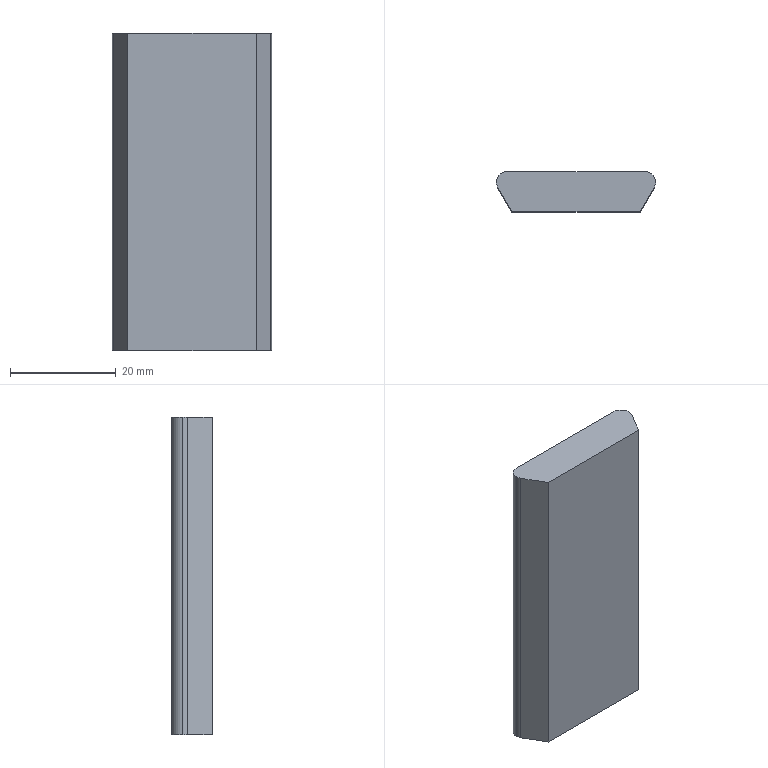Part | STEP file | 101000007812 | 1 solid | 10 faces | box 30.072 x 7.6 x 60 mm | volume 12718 mm3 | plane 6 | cylinder 4 | commonest cylinder face diameters 4 x4
STEP:
#1=CARTESIAN_POINT('',(10.458,8.,60.));
#2=VERTEX_POINT('',#1);
#3=CARTESIAN_POINT('',(10.726,7.,60.));
#4=VERTEX_POINT('',#3);
#5=CARTESIAN_POINT('',(12.458,8.,60.));
#6=DIRECTION('',(0.,0.,-1.));
#7=AXIS2_PLACEMENT_3D('',#5,#6,$);
#8=CIRCLE('',#7,2.);
#9=EDGE_CURVE('',#2,#4,#8,.F.);
#10=ORIENTED_EDGE('',*,*,#9,.F.);
#11=CARTESIAN_POINT('',(10.458,8.,0.));
#12=VERTEX_POINT('',#11);
#13=CARTESIAN_POINT('',(10.458,8.,60.));
#14=DIRECTION('',(0.,0.,-1.));
#15=VECTOR('',#14,1.);
#16=LINE('',#13,#15);
#17=EDGE_CURVE('',#2,#12,#16,.T.);
#18=ORIENTED_EDGE('',*,*,#17,.T.);
#19=CARTESIAN_POINT('',(10.726,7.,0.));
#20=VERTEX_POINT('',#19);
#21=CARTESIAN_POINT('',(12.458,8.,0.));
#22=DIRECTION('',(0.,0.,-1.));
#23=AXIS2_PLACEMENT_3D('',#21,#22,$);
#24=CIRCLE('',#23,2.);
#25=EDGE_CURVE('',#20,#12,#24,.T.);
#26=ORIENTED_EDGE('',*,*,#25,.F.);
#27=CARTESIAN_POINT('',(10.726,7.,60.));
#28=DIRECTION('',(0.,0.,-1.));
#29=VECTOR('',#28,1.);
#30=LINE('',#27,#29);
#31=EDGE_CURVE('',#4,#20,#30,.T.);
#32=ORIENTED_EDGE('',*,*,#31,.F.);
#33=EDGE_LOOP('',(#10,#18,#26,#32));
#34=FACE_OUTER_BOUND('',#33,.T.);
#35=CARTESIAN_POINT('',(12.458,8.,60.));
#36=DIRECTION('',(0.,0.,-1.));
#37=DIRECTION('',(1.,0.,0.));
#38=AXIS2_PLACEMENT_3D('',#35,#36,#37);
#39=CYLINDRICAL_SURFACE('',#38,2.);
#40=ADVANCED_FACE('',(#34),#39,.T.);
#41=CARTESIAN_POINT('',(37.606,2.4,60.));
#42=VERTEX_POINT('',#41);
#43=CARTESIAN_POINT('',(13.382,2.4,60.));
#44=VERTEX_POINT('',#43);
#45=CARTESIAN_POINT('',(25.494,2.4,60.));
#46=DIRECTION('',(-1.,0.,0.));
#47=VECTOR('',#46,1.);
#48=LINE('',#45,#47);
#49=EDGE_CURVE('',#42,#44,#48,.T.);
#50=ORIENTED_EDGE('',*,*,#49,.F.);
#51=CARTESIAN_POINT('',(40.262,7.,60.));
#52=VERTEX_POINT('',#51);
#53=CARTESIAN_POINT('',(38.934,4.7,60.));
#54=DIRECTION('',(0.5,0.866,0.));
#55=VECTOR('',#54,1.);
#56=LINE('',#53,#55);
#57=EDGE_CURVE('',#42,#52,#56,.T.);
#58=ORIENTED_EDGE('',*,*,#57,.T.);
#59=CARTESIAN_POINT('',(40.53,8.,60.));
#60=VERTEX_POINT('',#59);
#61=CARTESIAN_POINT('',(38.53,8.,60.));
#62=DIRECTION('',(0.,0.,1.));
#63=AXIS2_PLACEMENT_3D('',#61,#62,$);
#64=CIRCLE('',#63,2.);
#65=EDGE_CURVE('',#52,#60,#64,.T.);
#66=ORIENTED_EDGE('',*,*,#65,.T.);
#67=CARTESIAN_POINT('',(38.53,10.,60.));
#68=VERTEX_POINT('',#67);
#69=CARTESIAN_POINT('',(38.53,8.,60.));
#70=DIRECTION('',(0.,0.,1.));
#71=AXIS2_PLACEMENT_3D('',#69,#70,$);
#72=CIRCLE('',#71,2.);
#73=EDGE_CURVE('',#60,#68,#72,.T.);
#74=ORIENTED_EDGE('',*,*,#73,.T.);
#75=CARTESIAN_POINT('',(12.458,10.,60.));
#76=VERTEX_POINT('',#75);
#77=CARTESIAN_POINT('',(25.494,10.,60.));
#78=DIRECTION('',(-1.,0.,0.));
#79=VECTOR('',#78,1.);
#80=LINE('',#77,#79);
#81=EDGE_CURVE('',#68,#76,#80,.T.);
#82=ORIENTED_EDGE('',*,*,#81,.T.);
#83=CARTESIAN_POINT('',(12.458,8.,60.));
#84=DIRECTION('',(0.,0.,1.));
#85=AXIS2_PLACEMENT_3D('',#83,#84,$);
#86=CIRCLE('',#85,2.);
#87=EDGE_CURVE('',#76,#2,#86,.T.);
#88=ORIENTED_EDGE('',*,*,#87,.T.);
#89=ORIENTED_EDGE('',*,*,#9,.T.);
#90=CARTESIAN_POINT('',(12.054,4.7,60.));
#91=DIRECTION('',(0.5,-0.866,0.));
#92=VECTOR('',#91,1.);
#93=LINE('',#90,#92);
#94=EDGE_CURVE('',#4,#44,#93,.T.);
#95=ORIENTED_EDGE('',*,*,#94,.T.);
#96=EDGE_LOOP('',(#50,#58,#66,#74,#82,#88,#89,#95));
#97=FACE_OUTER_BOUND('',#96,.T.);
#98=CARTESIAN_POINT('',(36.22,0.,60.));
#99=DIRECTION('',(0.,0.,1.));
#100=DIRECTION('',(1.,0.,0.));
#101=AXIS2_PLACEMENT_3D('',#98,#99,#100);
#102=PLANE('',#101);
#103=ADVANCED_FACE('',(#97),#102,.T.);
#104=ORIENTED_EDGE('',*,*,#17,.F.);
#105=ORIENTED_EDGE('',*,*,#87,.F.);
#106=CARTESIAN_POINT('',(12.458,10.,0.));
#107=VERTEX_POINT('',#106);
#108=CARTESIAN_POINT('',(12.458,10.,60.));
#109=DIRECTION('',(0.,0.,-1.));
#110=VECTOR('',#109,1.);
#111=LINE('',#108,#110);
#112=EDGE_CURVE('',#107,#76,#111,.F.);
#113=ORIENTED_EDGE('',*,*,#112,.F.);
#114=CARTESIAN_POINT('',(12.458,8.,0.));
#115=DIRECTION('',(0.,0.,-1.));
#116=AXIS2_PLACEMENT_3D('',#114,#115,$);
#117=CIRCLE('',#116,2.);
#118=EDGE_CURVE('',#12,#107,#117,.T.);
#119=ORIENTED_EDGE('',*,*,#118,.F.);
#120=EDGE_LOOP('',(#104,#105,#113,#119));
#121=FACE_OUTER_BOUND('',#120,.T.);
#122=CARTESIAN_POINT('',(12.458,8.,60.));
#123=DIRECTION('',(0.,0.,-1.));
#124=DIRECTION('',(-1.,0.,0.));
#125=AXIS2_PLACEMENT_3D('',#122,#123,#124);
#126=CYLINDRICAL_SURFACE('',#125,2.);
#127=ADVANCED_FACE('',(#121),#126,.T.);
#128=CARTESIAN_POINT('',(37.606,2.4,0.));
#129=VERTEX_POINT('',#128);
#130=CARTESIAN_POINT('',(40.262,7.,0.));
#131=VERTEX_POINT('',#130);
#132=CARTESIAN_POINT('',(38.934,4.7,0.));
#133=DIRECTION('',(0.5,0.866,0.));
#134=VECTOR('',#133,1.);
#135=LINE('',#132,#134);
#136=EDGE_CURVE('',#129,#131,#135,.T.);
#137=ORIENTED_EDGE('',*,*,#136,.F.);
#138=CARTESIAN_POINT('',(13.382,2.4,0.));
#139=VERTEX_POINT('',#138);
#140=CARTESIAN_POINT('',(25.494,2.4,0.));
#141=DIRECTION('',(-1.,0.,0.));
#142=VECTOR('',#141,1.);
#143=LINE('',#140,#142);
#144=EDGE_CURVE('',#129,#139,#143,.T.);
#145=ORIENTED_EDGE('',*,*,#144,.T.);
#146=CARTESIAN_POINT('',(12.054,4.7,0.));
#147=DIRECTION('',(0.5,-0.866,0.));
#148=VECTOR('',#147,1.);
#149=LINE('',#146,#148);
#150=EDGE_CURVE('',#20,#139,#149,.T.);
#151=ORIENTED_EDGE('',*,*,#150,.F.);
#152=ORIENTED_EDGE('',*,*,#25,.T.);
#153=ORIENTED_EDGE('',*,*,#118,.T.);
#154=CARTESIAN_POINT('',(38.53,10.,0.));
#155=VERTEX_POINT('',#154);
#156=CARTESIAN_POINT('',(25.494,10.,0.));
#157=DIRECTION('',(-1.,0.,0.));
#158=VECTOR('',#157,1.);
#159=LINE('',#156,#158);
#160=EDGE_CURVE('',#155,#107,#159,.T.);
#161=ORIENTED_EDGE('',*,*,#160,.F.);
#162=CARTESIAN_POINT('',(40.53,8.,0.));
#163=VERTEX_POINT('',#162);
#164=CARTESIAN_POINT('',(38.53,10.,0.));
#165=CARTESIAN_POINT('',(38.737,10.,0.));
#166=CARTESIAN_POINT('',(38.945,9.973,0.));
#167=CARTESIAN_POINT('',(39.148,9.919,0.));
#168=CARTESIAN_POINT('',(39.536,9.759,0.));
#169=CARTESIAN_POINT('',(39.87,9.506,0.));
#170=CARTESIAN_POINT('',(40.02,9.358,0.));
#171=CARTESIAN_POINT('',(40.277,9.027,0.));
#172=CARTESIAN_POINT('',(40.441,8.642,0.));
#173=CARTESIAN_POINT('',(40.498,8.439,0.));
#174=CARTESIAN_POINT('',(40.528,8.227,0.));
#175=CARTESIAN_POINT('',(40.53,8.014,0.));
#176=CARTESIAN_POINT('',(40.53,8.01,0.));
#177=CARTESIAN_POINT('',(40.53,8.005,0.));
#178=CARTESIAN_POINT('',(40.53,8.,0.));
#179=B_SPLINE_CURVE_WITH_KNOTS('',5,(#164,#165,#166,#167,#168,#169,#170,#171,#172,#173,#174,#175,#176,#177,#178),.UNSPECIFIED.,.F.,.U.,(6,3,3,3,6),(0.,1.47,2.939,4.409,4.443),.UNSPECIFIED.);
#180=EDGE_CURVE('',#155,#163,#179,.T.);
#181=ORIENTED_EDGE('',*,*,#180,.T.);
#182=CARTESIAN_POINT('',(40.53,8.,0.));
#183=CARTESIAN_POINT('',(40.53,7.797,0.));
#184=CARTESIAN_POINT('',(40.504,7.594,0.));
#185=CARTESIAN_POINT('',(40.452,7.395,0.));
#186=CARTESIAN_POINT('',(40.374,7.199,0.));
#187=CARTESIAN_POINT('',(40.271,7.017,0.));
#188=CARTESIAN_POINT('',(40.268,7.011,0.));
#189=CARTESIAN_POINT('',(40.265,7.006,0.));
#190=CARTESIAN_POINT('',(40.262,7.,0.));
#191=B_SPLINE_CURVE_WITH_KNOTS('',5,(#182,#183,#184,#185,#186,#187,#188,#189,#190),.UNSPECIFIED.,.F.,.U.,(6,3,6),(4.443,5.879,5.924),.UNSPECIFIED.);
#192=EDGE_CURVE('',#163,#131,#191,.T.);
#193=ORIENTED_EDGE('',*,*,#192,.T.);
#194=EDGE_LOOP('',(#137,#145,#151,#152,#153,#161,#181,#193));
#195=FACE_OUTER_BOUND('',#194,.T.);
#196=CARTESIAN_POINT('',(36.22,0.,0.));
#197=DIRECTION('',(0.,0.,1.));
#198=DIRECTION('',(1.,0.,0.));
#199=AXIS2_PLACEMENT_3D('',#196,#197,#198);
#200=PLANE('',#199);
#201=ADVANCED_FACE('',(#195),#200,.F.);
#202=ORIENTED_EDGE('',*,*,#150,.T.);
#203=CARTESIAN_POINT('',(13.382,2.4,30.));
#204=DIRECTION('',(0.,0.,1.));
#205=VECTOR('',#204,1.);
#206=LINE('',#203,#205);
#207=EDGE_CURVE('',#139,#44,#206,.T.);
#208=ORIENTED_EDGE('',*,*,#207,.T.);
#209=ORIENTED_EDGE('',*,*,#94,.F.);
#210=ORIENTED_EDGE('',*,*,#31,.T.);
#211=EDGE_LOOP('',(#202,#208,#209,#210));
#212=FACE_OUTER_BOUND('',#211,.T.);
#213=CARTESIAN_POINT('',(14.767,0.,60.));
#214=DIRECTION('',(0.866,0.5,0.));
#215=DIRECTION('',(-0.5,0.866,0.));
#216=AXIS2_PLACEMENT_3D('',#213,#214,#215);
#217=PLANE('',#216);
#218=ADVANCED_FACE('',(#212),#217,.F.);
#219=ORIENTED_EDGE('',*,*,#49,.T.);
#220=ORIENTED_EDGE('',*,*,#207,.F.);
#221=ORIENTED_EDGE('',*,*,#144,.F.);
#222=CARTESIAN_POINT('',(37.606,2.4,30.));
#223=DIRECTION('',(0.,0.,-1.));
#224=VECTOR('',#223,1.);
#225=LINE('',#222,#224);
#226=EDGE_CURVE('',#42,#129,#225,.T.);
#227=ORIENTED_EDGE('',*,*,#226,.F.);
#228=EDGE_LOOP('',(#219,#220,#221,#227));
#229=FACE_OUTER_BOUND('',#228,.T.);
#230=CARTESIAN_POINT('',(10.494,2.4,0.));
#231=DIRECTION('',(0.,1.,0.));
#232=DIRECTION('',(-1.,0.,0.));
#233=AXIS2_PLACEMENT_3D('',#230,#231,#232);
#234=PLANE('',#233);
#235=ADVANCED_FACE('',(#229),#234,.F.);
#236=ORIENTED_EDGE('',*,*,#57,.F.);
#237=ORIENTED_EDGE('',*,*,#226,.T.);
#238=ORIENTED_EDGE('',*,*,#136,.T.);
#239=CARTESIAN_POINT('',(40.262,7.,30.));
#240=DIRECTION('',(0.,0.,1.));
#241=VECTOR('',#240,1.);
#242=LINE('',#239,#241);
#243=EDGE_CURVE('',#131,#52,#242,.T.);
#244=ORIENTED_EDGE('',*,*,#243,.T.);
#245=EDGE_LOOP('',(#236,#237,#238,#244));
#246=FACE_OUTER_BOUND('',#245,.T.);
#247=CARTESIAN_POINT('',(36.22,0.,60.));
#248=DIRECTION('',(-0.866,0.5,0.));
#249=DIRECTION('',(-0.5,-0.866,0.));
#250=AXIS2_PLACEMENT_3D('',#247,#248,#249);
#251=PLANE('',#250);
#252=ADVANCED_FACE('',(#246),#251,.F.);
#253=CARTESIAN_POINT('',(40.53,8.,60.));
#254=DIRECTION('',(0.,0.,-1.));
#255=VECTOR('',#254,1.);
#256=LINE('',#253,#255);
#257=EDGE_CURVE('',#60,#163,#256,.T.);
#258=ORIENTED_EDGE('',*,*,#257,.F.);
#259=ORIENTED_EDGE('',*,*,#65,.F.);
#260=ORIENTED_EDGE('',*,*,#243,.F.);
#261=ORIENTED_EDGE('',*,*,#192,.F.);
#262=EDGE_LOOP('',(#258,#259,#260,#261));
#263=FACE_OUTER_BOUND('',#262,.T.);
#264=CARTESIAN_POINT('',(38.53,8.,60.));
#265=DIRECTION('',(0.,0.,-1.));
#266=DIRECTION('',(1.,0.,0.));
#267=AXIS2_PLACEMENT_3D('',#264,#265,#266);
#268=CYLINDRICAL_SURFACE('',#267,2.);
#269=ADVANCED_FACE('',(#263),#268,.T.);
#270=ORIENTED_EDGE('',*,*,#257,.T.);
#271=ORIENTED_EDGE('',*,*,#180,.F.);
#272=CARTESIAN_POINT('',(38.53,10.,60.));
#273=DIRECTION('',(0.,0.,-1.));
#274=VECTOR('',#273,1.);
#275=LINE('',#272,#274);
#276=EDGE_CURVE('',#68,#155,#275,.T.);
#277=ORIENTED_EDGE('',*,*,#276,.F.);
#278=ORIENTED_EDGE('',*,*,#73,.F.);
#279=EDGE_LOOP('',(#270,#271,#277,#278));
#280=FACE_OUTER_BOUND('',#279,.T.);
#281=CARTESIAN_POINT('',(38.53,8.,60.));
#282=DIRECTION('',(0.,0.,-1.));
#283=DIRECTION('',(-1.,0.,0.));
#284=AXIS2_PLACEMENT_3D('',#281,#282,#283);
#285=CYLINDRICAL_SURFACE('',#284,2.);
#286=ADVANCED_FACE('',(#280),#285,.T.);
#287=ORIENTED_EDGE('',*,*,#81,.F.);
#288=ORIENTED_EDGE('',*,*,#276,.T.);
#289=ORIENTED_EDGE('',*,*,#160,.T.);
#290=ORIENTED_EDGE('',*,*,#112,.T.);
#291=EDGE_LOOP('',(#287,#288,#289,#290));
#292=FACE_OUTER_BOUND('',#291,.T.);
#293=CARTESIAN_POINT('',(8.994,10.,60.));
#294=DIRECTION('',(0.,-1.,0.));
#295=DIRECTION('',(1.,0.,0.));
#296=AXIS2_PLACEMENT_3D('',#293,#294,#295);
#297=PLANE('',#296);
#298=ADVANCED_FACE('',(#292),#297,.F.);
#299=CLOSED_SHELL('',(#40,#103,#127,#201,#218,#235,#252,#269,#286,#298));
#300=MANIFOLD_SOLID_BREP('',#299);
#301=(LENGTH_UNIT()NAMED_UNIT(*)SI_UNIT(.MILLI.,.METRE.));
#302=UNCERTAINTY_MEASURE_WITH_UNIT(LENGTH_MEASURE(0.005),#301,'','');
#303=(NAMED_UNIT(*)PLANE_ANGLE_UNIT()SI_UNIT($,.RADIAN.));
#304=(NAMED_UNIT(*)SI_UNIT($,.STERADIAN.)SOLID_ANGLE_UNIT());
#305=(GEOMETRIC_REPRESENTATION_CONTEXT(3)GLOBAL_UNCERTAINTY_ASSIGNED_CONTEXT((#302))GLOBAL_UNIT_ASSIGNED_CONTEXT((#301,#303,#304))REPRESENTATION_CONTEXT('',''));
#306=ADVANCED_BREP_SHAPE_REPRESENTATION('',(#300),#305);